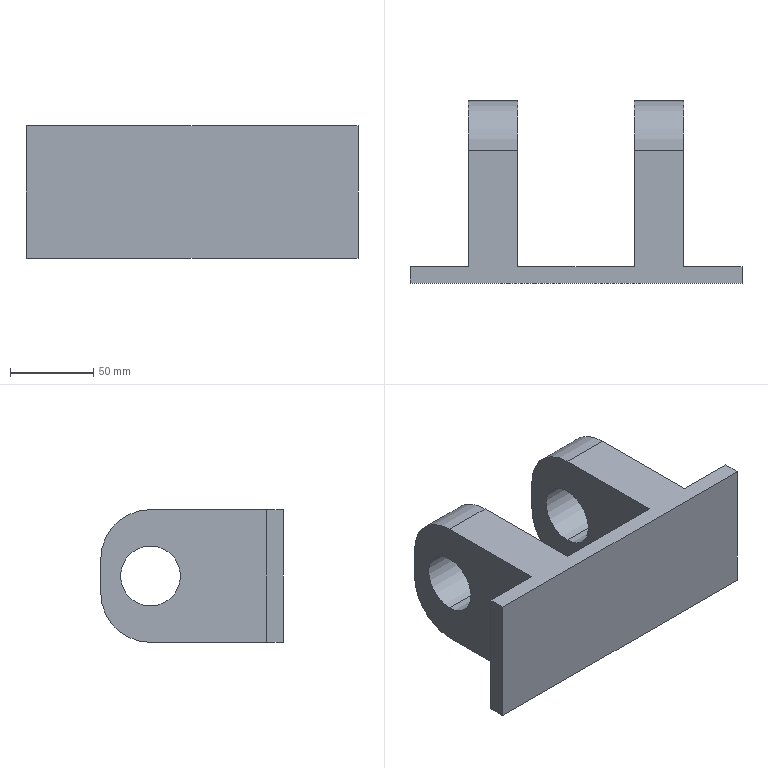Part | STEP file | Traction rod base | 1 solid | 22 faces | box 200 x 110 x 80 mm | volume 555750 mm3 | plane 14 | cylinder 8 | commonest cylinder face diameters 36 x4 60 x4
STEP:
#1=CARTESIAN_POINT('',(65.,80.,18.));
#2=VERTEX_POINT('',#1);
#3=CARTESIAN_POINT('',(65.,80.,-18.));
#4=VERTEX_POINT('',#3);
#5=CARTESIAN_POINT('',(65.,80.,0.));
#6=DIRECTION('',(1.,0.,0.));
#7=DIRECTION('',(0.,0.,-1.));
#8=AXIS2_PLACEMENT_3D('',#5,#6,#7);
#9=CIRCLE('',#8,18.);
#10=EDGE_CURVE('',#2,#4,#9,.T.);
#11=ORIENTED_EDGE('',*,*,#10,.T.);
#12=CARTESIAN_POINT('',(35.,80.,-18.));
#13=VERTEX_POINT('',#12);
#14=CARTESIAN_POINT('',(100.001,80.,-18.));
#15=DIRECTION('',(-1.,0.,0.));
#16=VECTOR('',#15,1000.);
#17=LINE('',#14,#16);
#18=EDGE_CURVE('',#4,#13,#17,.T.);
#19=ORIENTED_EDGE('',*,*,#18,.T.);
#20=CARTESIAN_POINT('',(35.,80.,18.));
#21=VERTEX_POINT('',#20);
#22=CARTESIAN_POINT('',(35.,80.,0.));
#23=DIRECTION('',(1.,0.,0.));
#24=DIRECTION('',(0.,0.,-1.));
#25=AXIS2_PLACEMENT_3D('',#22,#23,#24);
#26=CIRCLE('',#25,18.);
#27=EDGE_CURVE('',#21,#13,#26,.T.);
#28=ORIENTED_EDGE('',*,*,#27,.F.);
#29=CARTESIAN_POINT('',(100.001,80.,18.));
#30=DIRECTION('',(-1.,0.,0.));
#31=VECTOR('',#30,1000.);
#32=LINE('',#29,#31);
#33=EDGE_CURVE('',#2,#21,#32,.T.);
#34=ORIENTED_EDGE('',*,*,#33,.F.);
#35=EDGE_LOOP('',(#11,#19,#28,#34));
#36=FACE_OUTER_BOUND('',#35,.T.);
#37=CARTESIAN_POINT('',(100.001,80.,0.));
#38=DIRECTION('',(-1.,0.,0.));
#39=DIRECTION('',(0.,0.,1.));
#40=AXIS2_PLACEMENT_3D('',#37,#38,#39);
#41=CYLINDRICAL_SURFACE('',#40,18.);
#42=ADVANCED_FACE('',(#36),#41,.F.);
#43=CARTESIAN_POINT('',(-65.,80.,-18.));
#44=VERTEX_POINT('',#43);
#45=CARTESIAN_POINT('',(-65.,80.,18.));
#46=VERTEX_POINT('',#45);
#47=CARTESIAN_POINT('',(-65.,80.,0.));
#48=DIRECTION('',(-1.,0.,0.));
#49=DIRECTION('',(0.,0.,-1.));
#50=AXIS2_PLACEMENT_3D('',#47,#48,#49);
#51=CIRCLE('',#50,18.);
#52=EDGE_CURVE('',#44,#46,#51,.T.);
#53=ORIENTED_EDGE('',*,*,#52,.T.);
#54=CARTESIAN_POINT('',(-35.,80.,18.));
#55=VERTEX_POINT('',#54);
#56=CARTESIAN_POINT('',(-100.001,80.,18.));
#57=DIRECTION('',(1.,0.,0.));
#58=VECTOR('',#57,1000.);
#59=LINE('',#56,#58);
#60=EDGE_CURVE('',#46,#55,#59,.T.);
#61=ORIENTED_EDGE('',*,*,#60,.T.);
#62=CARTESIAN_POINT('',(-35.,80.,-18.));
#63=VERTEX_POINT('',#62);
#64=CARTESIAN_POINT('',(-35.,80.,0.));
#65=DIRECTION('',(1.,0.,0.));
#66=DIRECTION('',(0.,0.,-1.));
#67=AXIS2_PLACEMENT_3D('',#64,#65,#66);
#68=CIRCLE('',#67,18.);
#69=EDGE_CURVE('',#55,#63,#68,.T.);
#70=ORIENTED_EDGE('',*,*,#69,.T.);
#71=CARTESIAN_POINT('',(-100.001,80.,-18.));
#72=DIRECTION('',(1.,0.,0.));
#73=VECTOR('',#72,1000.);
#74=LINE('',#71,#73);
#75=EDGE_CURVE('',#44,#63,#74,.T.);
#76=ORIENTED_EDGE('',*,*,#75,.F.);
#77=EDGE_LOOP('',(#53,#61,#70,#76));
#78=FACE_OUTER_BOUND('',#77,.T.);
#79=CARTESIAN_POINT('',(-100.001,80.,0.));
#80=DIRECTION('',(1.,0.,0.));
#81=DIRECTION('',(0.,0.,-1.));
#82=AXIS2_PLACEMENT_3D('',#79,#80,#81);
#83=CYLINDRICAL_SURFACE('',#82,18.);
#84=ADVANCED_FACE('',(#78),#83,.F.);
#85=CARTESIAN_POINT('',(65.,10.,-40.));
#86=VERTEX_POINT('',#85);
#87=CARTESIAN_POINT('',(65.,10.,40.));
#88=VERTEX_POINT('',#87);
#89=CARTESIAN_POINT('',(65.,10.,-40.));
#90=DIRECTION('',(0.,0.,1.));
#91=VECTOR('',#90,1000.);
#92=LINE('',#89,#91);
#93=EDGE_CURVE('',#86,#88,#92,.T.);
#94=ORIENTED_EDGE('',*,*,#93,.T.);
#95=CARTESIAN_POINT('',(100.,10.,40.));
#96=VERTEX_POINT('',#95);
#97=CARTESIAN_POINT('',(-100.,10.,40.));
#98=DIRECTION('',(1.,0.,0.));
#99=VECTOR('',#98,1000.);
#100=LINE('',#97,#99);
#101=EDGE_CURVE('',#88,#96,#100,.T.);
#102=ORIENTED_EDGE('',*,*,#101,.T.);
#103=CARTESIAN_POINT('',(100.,10.,-40.));
#104=VERTEX_POINT('',#103);
#105=CARTESIAN_POINT('',(100.,10.,-40.));
#106=DIRECTION('',(0.,0.,1.));
#107=VECTOR('',#106,1000.);
#108=LINE('',#105,#107);
#109=EDGE_CURVE('',#104,#96,#108,.T.);
#110=ORIENTED_EDGE('',*,*,#109,.F.);
#111=CARTESIAN_POINT('',(-100.,10.,-40.));
#112=DIRECTION('',(1.,0.,0.));
#113=VECTOR('',#112,1000.);
#114=LINE('',#111,#113);
#115=EDGE_CURVE('',#86,#104,#114,.T.);
#116=ORIENTED_EDGE('',*,*,#115,.F.);
#117=EDGE_LOOP('',(#94,#102,#110,#116));
#118=FACE_OUTER_BOUND('',#117,.T.);
#119=CARTESIAN_POINT('',(0.,10.,0.));
#120=DIRECTION('',(0.,1.,0.));
#121=DIRECTION('',(0.,0.,1.));
#122=AXIS2_PLACEMENT_3D('',#119,#120,#121);
#123=PLANE('',#122);
#124=ADVANCED_FACE('',(#118),#123,.T.);
#125=CARTESIAN_POINT('',(-65.,10.,-40.));
#126=VERTEX_POINT('',#125);
#127=CARTESIAN_POINT('',(-65.,10.,40.));
#128=VERTEX_POINT('',#127);
#129=CARTESIAN_POINT('',(-65.,10.,-40.));
#130=DIRECTION('',(0.,0.,1.));
#131=VECTOR('',#130,1000.);
#132=LINE('',#129,#131);
#133=EDGE_CURVE('',#126,#128,#132,.T.);
#134=ORIENTED_EDGE('',*,*,#133,.F.);
#135=CARTESIAN_POINT('',(-100.,10.,-40.));
#136=VERTEX_POINT('',#135);
#137=CARTESIAN_POINT('',(-100.,10.,-40.));
#138=DIRECTION('',(1.,0.,0.));
#139=VECTOR('',#138,1000.);
#140=LINE('',#137,#139);
#141=EDGE_CURVE('',#136,#126,#140,.T.);
#142=ORIENTED_EDGE('',*,*,#141,.F.);
#143=CARTESIAN_POINT('',(-100.,10.,40.));
#144=VERTEX_POINT('',#143);
#145=CARTESIAN_POINT('',(-100.,10.,-40.));
#146=DIRECTION('',(0.,0.,1.));
#147=VECTOR('',#146,1000.);
#148=LINE('',#145,#147);
#149=EDGE_CURVE('',#136,#144,#148,.T.);
#150=ORIENTED_EDGE('',*,*,#149,.T.);
#151=CARTESIAN_POINT('',(-100.,10.,40.));
#152=DIRECTION('',(1.,0.,0.));
#153=VECTOR('',#152,1000.);
#154=LINE('',#151,#153);
#155=EDGE_CURVE('',#144,#128,#154,.T.);
#156=ORIENTED_EDGE('',*,*,#155,.T.);
#157=EDGE_LOOP('',(#134,#142,#150,#156));
#158=FACE_OUTER_BOUND('',#157,.T.);
#159=CARTESIAN_POINT('',(0.,10.,0.));
#160=DIRECTION('',(0.,1.,0.));
#161=DIRECTION('',(0.,0.,1.));
#162=AXIS2_PLACEMENT_3D('',#159,#160,#161);
#163=PLANE('',#162);
#164=ADVANCED_FACE('',(#158),#163,.T.);
#165=CARTESIAN_POINT('',(-100.,0.,-40.));
#166=VERTEX_POINT('',#165);
#167=CARTESIAN_POINT('',(-100.,0.,40.));
#168=VERTEX_POINT('',#167);
#169=CARTESIAN_POINT('',(-100.,0.,-40.));
#170=DIRECTION('',(0.,0.,1.));
#171=VECTOR('',#170,1000.);
#172=LINE('',#169,#171);
#173=EDGE_CURVE('',#166,#168,#172,.T.);
#174=ORIENTED_EDGE('',*,*,#173,.T.);
#175=CARTESIAN_POINT('',(-100.,10.,40.));
#176=DIRECTION('',(0.,-1.,0.));
#177=VECTOR('',#176,1000.);
#178=LINE('',#175,#177);
#179=EDGE_CURVE('',#144,#168,#178,.T.);
#180=ORIENTED_EDGE('',*,*,#179,.F.);
#181=ORIENTED_EDGE('',*,*,#149,.F.);
#182=CARTESIAN_POINT('',(-100.,10.,-40.));
#183=DIRECTION('',(0.,-1.,0.));
#184=VECTOR('',#183,1000.);
#185=LINE('',#182,#184);
#186=EDGE_CURVE('',#136,#166,#185,.T.);
#187=ORIENTED_EDGE('',*,*,#186,.T.);
#188=EDGE_LOOP('',(#174,#180,#181,#187));
#189=FACE_OUTER_BOUND('',#188,.T.);
#190=CARTESIAN_POINT('',(-100.,10.,-40.));
#191=DIRECTION('',(1.,0.,0.));
#192=DIRECTION('',(0.,0.,-1.));
#193=AXIS2_PLACEMENT_3D('',#190,#191,#192);
#194=PLANE('',#193);
#195=ADVANCED_FACE('',(#189),#194,.F.);
#196=CARTESIAN_POINT('',(65.,80.,40.));
#197=VERTEX_POINT('',#196);
#198=CARTESIAN_POINT('',(65.,110.,40.));
#199=DIRECTION('',(0.,-1.,0.));
#200=VECTOR('',#199,1000.);
#201=LINE('',#198,#200);
#202=EDGE_CURVE('',#197,#88,#201,.T.);
#203=ORIENTED_EDGE('',*,*,#202,.F.);
#204=CARTESIAN_POINT('',(35.,80.,40.));
#205=VERTEX_POINT('',#204);
#206=CARTESIAN_POINT('',(35.,80.,40.));
#207=DIRECTION('',(-1.,0.,0.));
#208=VECTOR('',#207,1000.);
#209=LINE('',#206,#208);
#210=EDGE_CURVE('',#197,#205,#209,.T.);
#211=ORIENTED_EDGE('',*,*,#210,.T.);
#212=CARTESIAN_POINT('',(35.,10.,40.));
#213=VERTEX_POINT('',#212);
#214=CARTESIAN_POINT('',(35.,110.,40.));
#215=DIRECTION('',(0.,-1.,0.));
#216=VECTOR('',#215,1000.);
#217=LINE('',#214,#216);
#218=EDGE_CURVE('',#205,#213,#217,.T.);
#219=ORIENTED_EDGE('',*,*,#218,.T.);
#220=CARTESIAN_POINT('',(-35.,10.,40.));
#221=VERTEX_POINT('',#220);
#222=CARTESIAN_POINT('',(-100.,10.,40.));
#223=DIRECTION('',(1.,0.,0.));
#224=VECTOR('',#223,1000.);
#225=LINE('',#222,#224);
#226=EDGE_CURVE('',#221,#213,#225,.T.);
#227=ORIENTED_EDGE('',*,*,#226,.F.);
#228=CARTESIAN_POINT('',(-35.,80.,40.));
#229=VERTEX_POINT('',#228);
#230=CARTESIAN_POINT('',(-35.,110.,40.));
#231=DIRECTION('',(0.,-1.,0.));
#232=VECTOR('',#231,1000.);
#233=LINE('',#230,#232);
#234=EDGE_CURVE('',#229,#221,#233,.T.);
#235=ORIENTED_EDGE('',*,*,#234,.F.);
#236=CARTESIAN_POINT('',(-65.,80.,40.));
#237=VERTEX_POINT('',#236);
#238=CARTESIAN_POINT('',(-65.,80.,40.));
#239=DIRECTION('',(-1.,0.,0.));
#240=VECTOR('',#239,1000.);
#241=LINE('',#238,#240);
#242=EDGE_CURVE('',#229,#237,#241,.T.);
#243=ORIENTED_EDGE('',*,*,#242,.T.);
#244=CARTESIAN_POINT('',(-65.,110.,40.));
#245=DIRECTION('',(0.,-1.,0.));
#246=VECTOR('',#245,1000.);
#247=LINE('',#244,#246);
#248=EDGE_CURVE('',#237,#128,#247,.T.);
#249=ORIENTED_EDGE('',*,*,#248,.T.);
#250=ORIENTED_EDGE('',*,*,#155,.F.);
#251=ORIENTED_EDGE('',*,*,#179,.T.);
#252=CARTESIAN_POINT('',(100.,0.,40.));
#253=VERTEX_POINT('',#252);
#254=CARTESIAN_POINT('',(-100.,0.,40.));
#255=DIRECTION('',(1.,0.,0.));
#256=VECTOR('',#255,1000.);
#257=LINE('',#254,#256);
#258=EDGE_CURVE('',#168,#253,#257,.T.);
#259=ORIENTED_EDGE('',*,*,#258,.T.);
#260=CARTESIAN_POINT('',(100.,10.,40.));
#261=DIRECTION('',(0.,-1.,0.));
#262=VECTOR('',#261,1000.);
#263=LINE('',#260,#262);
#264=EDGE_CURVE('',#96,#253,#263,.T.);
#265=ORIENTED_EDGE('',*,*,#264,.F.);
#266=ORIENTED_EDGE('',*,*,#101,.F.);
#267=EDGE_LOOP('',(#203,#211,#219,#227,#235,#243,#249,#250,#251,#259,#265,#266));
#268=FACE_OUTER_BOUND('',#267,.T.);
#269=CARTESIAN_POINT('',(-100.,10.,40.));
#270=DIRECTION('',(0.,0.,-1.));
#271=DIRECTION('',(-1.,0.,0.));
#272=AXIS2_PLACEMENT_3D('',#269,#270,#271);
#273=PLANE('',#272);
#274=ADVANCED_FACE('',(#268),#273,.F.);
#275=CARTESIAN_POINT('',(100.,0.,-40.));
#276=VERTEX_POINT('',#275);
#277=CARTESIAN_POINT('',(100.,0.,-40.));
#278=DIRECTION('',(0.,0.,1.));
#279=VECTOR('',#278,1000.);
#280=LINE('',#277,#279);
#281=EDGE_CURVE('',#276,#253,#280,.T.);
#282=ORIENTED_EDGE('',*,*,#281,.F.);
#283=CARTESIAN_POINT('',(100.,10.,-40.));
#284=DIRECTION('',(0.,-1.,0.));
#285=VECTOR('',#284,1000.);
#286=LINE('',#283,#285);
#287=EDGE_CURVE('',#104,#276,#286,.T.);
#288=ORIENTED_EDGE('',*,*,#287,.F.);
#289=ORIENTED_EDGE('',*,*,#109,.T.);
#290=ORIENTED_EDGE('',*,*,#264,.T.);
#291=EDGE_LOOP('',(#282,#288,#289,#290));
#292=FACE_OUTER_BOUND('',#291,.T.);
#293=CARTESIAN_POINT('',(100.,10.,-40.));
#294=DIRECTION('',(1.,0.,0.));
#295=DIRECTION('',(0.,0.,-1.));
#296=AXIS2_PLACEMENT_3D('',#293,#294,#295);
#297=PLANE('',#296);
#298=ADVANCED_FACE('',(#292),#297,.T.);
#299=CARTESIAN_POINT('',(35.,80.,-40.));
#300=VERTEX_POINT('',#299);
#301=CARTESIAN_POINT('',(35.,10.,-40.));
#302=VERTEX_POINT('',#301);
#303=CARTESIAN_POINT('',(35.,110.,-40.));
#304=DIRECTION('',(0.,-1.,0.));
#305=VECTOR('',#304,1000.);
#306=LINE('',#303,#305);
#307=EDGE_CURVE('',#300,#302,#306,.T.);
#308=ORIENTED_EDGE('',*,*,#307,.F.);
#309=CARTESIAN_POINT('',(65.,80.,-40.));
#310=VERTEX_POINT('',#309);
#311=CARTESIAN_POINT('',(-100.,80.,-40.));
#312=DIRECTION('',(1.,0.,0.));
#313=VECTOR('',#312,1000.);
#314=LINE('',#311,#313);
#315=EDGE_CURVE('',#300,#310,#314,.T.);
#316=ORIENTED_EDGE('',*,*,#315,.T.);
#317=CARTESIAN_POINT('',(65.,110.,-40.));
#318=DIRECTION('',(0.,-1.,0.));
#319=VECTOR('',#318,1000.);
#320=LINE('',#317,#319);
#321=EDGE_CURVE('',#310,#86,#320,.T.);
#322=ORIENTED_EDGE('',*,*,#321,.T.);
#323=ORIENTED_EDGE('',*,*,#115,.T.);
#324=ORIENTED_EDGE('',*,*,#287,.T.);
#325=CARTESIAN_POINT('',(-100.,0.,-40.));
#326=DIRECTION('',(1.,0.,0.));
#327=VECTOR('',#326,1000.);
#328=LINE('',#325,#327);
#329=EDGE_CURVE('',#166,#276,#328,.T.);
#330=ORIENTED_EDGE('',*,*,#329,.F.);
#331=ORIENTED_EDGE('',*,*,#186,.F.);
#332=ORIENTED_EDGE('',*,*,#141,.T.);
#333=CARTESIAN_POINT('',(-65.,80.,-40.));
#334=VERTEX_POINT('',#333);
#335=CARTESIAN_POINT('',(-65.,110.,-40.));
#336=DIRECTION('',(0.,-1.,0.));
#337=VECTOR('',#336,1000.);
#338=LINE('',#335,#337);
#339=EDGE_CURVE('',#334,#126,#338,.T.);
#340=ORIENTED_EDGE('',*,*,#339,.F.);
#341=CARTESIAN_POINT('',(-35.,80.,-40.));
#342=VERTEX_POINT('',#341);
#343=CARTESIAN_POINT('',(-100.,80.,-40.));
#344=DIRECTION('',(1.,0.,0.));
#345=VECTOR('',#344,1000.);
#346=LINE('',#343,#345);
#347=EDGE_CURVE('',#334,#342,#346,.T.);
#348=ORIENTED_EDGE('',*,*,#347,.T.);
#349=CARTESIAN_POINT('',(-35.,10.,-40.));
#350=VERTEX_POINT('',#349);
#351=CARTESIAN_POINT('',(-35.,110.,-40.));
#352=DIRECTION('',(0.,-1.,0.));
#353=VECTOR('',#352,1000.);
#354=LINE('',#351,#353);
#355=EDGE_CURVE('',#342,#350,#354,.T.);
#356=ORIENTED_EDGE('',*,*,#355,.T.);
#357=CARTESIAN_POINT('',(-100.,10.,-40.));
#358=DIRECTION('',(1.,0.,0.));
#359=VECTOR('',#358,1000.);
#360=LINE('',#357,#359);
#361=EDGE_CURVE('',#350,#302,#360,.T.);
#362=ORIENTED_EDGE('',*,*,#361,.T.);
#363=EDGE_LOOP('',(#308,#316,#322,#323,#324,#330,#331,#332,#340,#348,#356,#362));
#364=FACE_OUTER_BOUND('',#363,.T.);
#365=CARTESIAN_POINT('',(-100.,10.,-40.));
#366=DIRECTION('',(0.,0.,-1.));
#367=DIRECTION('',(-1.,0.,0.));
#368=AXIS2_PLACEMENT_3D('',#365,#366,#367);
#369=PLANE('',#368);
#370=ADVANCED_FACE('',(#364),#369,.T.);
#371=CARTESIAN_POINT('',(35.,10.,-40.));
#372=DIRECTION('',(0.,0.,-1.));
#373=VECTOR('',#372,1000.);
#374=LINE('',#371,#373);
#375=EDGE_CURVE('',#213,#302,#374,.T.);
#376=ORIENTED_EDGE('',*,*,#375,.T.);
#377=ORIENTED_EDGE('',*,*,#361,.F.);
#378=CARTESIAN_POINT('',(-35.,10.,-40.));
#379=DIRECTION('',(0.,0.,-1.));
#380=VECTOR('',#379,1000.);
#381=LINE('',#378,#380);
#382=EDGE_CURVE('',#221,#350,#381,.T.);
#383=ORIENTED_EDGE('',*,*,#382,.F.);
#384=ORIENTED_EDGE('',*,*,#226,.T.);
#385=EDGE_LOOP('',(#376,#377,#383,#384));
#386=FACE_OUTER_BOUND('',#385,.T.);
#387=CARTESIAN_POINT('',(0.,10.,0.));
#388=DIRECTION('',(0.,1.,0.));
#389=DIRECTION('',(0.,0.,1.));
#390=AXIS2_PLACEMENT_3D('',#387,#388,#389);
#391=PLANE('',#390);
#392=ADVANCED_FACE('',(#386),#391,.T.);
#393=ORIENTED_EDGE('',*,*,#173,.F.);
#394=ORIENTED_EDGE('',*,*,#329,.T.);
#395=ORIENTED_EDGE('',*,*,#281,.T.);
#396=ORIENTED_EDGE('',*,*,#258,.F.);
#397=EDGE_LOOP('',(#393,#394,#395,#396));
#398=FACE_OUTER_BOUND('',#397,.T.);
#399=CARTESIAN_POINT('',(0.,0.,0.));
#400=DIRECTION('',(0.,1.,0.));
#401=DIRECTION('',(0.,0.,1.));
#402=AXIS2_PLACEMENT_3D('',#399,#400,#401);
#403=PLANE('',#402);
#404=ADVANCED_FACE('',(#398),#403,.F.);
#405=ORIENTED_EDGE('',*,*,#52,.F.);
#406=CARTESIAN_POINT('',(-65.,80.,0.));
#407=DIRECTION('',(-1.,0.,0.));
#408=DIRECTION('',(0.,0.,-1.));
#409=AXIS2_PLACEMENT_3D('',#406,#407,#408);
#410=CIRCLE('',#409,18.);
#411=EDGE_CURVE('',#46,#44,#410,.T.);
#412=ORIENTED_EDGE('',*,*,#411,.F.);
#413=EDGE_LOOP('',(#405,#412));
#414=FACE_BOUND('',#413,.T.);
#415=CARTESIAN_POINT('',(-65.,110.,-10.));
#416=VERTEX_POINT('',#415);
#417=CARTESIAN_POINT('',(-65.,110.,10.));
#418=VERTEX_POINT('',#417);
#419=CARTESIAN_POINT('',(-65.,110.,-40.));
#420=DIRECTION('',(0.,0.,1.));
#421=VECTOR('',#420,1000.);
#422=LINE('',#419,#421);
#423=EDGE_CURVE('',#416,#418,#422,.T.);
#424=ORIENTED_EDGE('',*,*,#423,.F.);
#425=CARTESIAN_POINT('',(-65.,80.,-10.));
#426=DIRECTION('',(-1.,0.,0.));
#427=DIRECTION('',(0.,0.,-1.));
#428=AXIS2_PLACEMENT_3D('',#425,#426,#427);
#429=CIRCLE('',#428,30.);
#430=EDGE_CURVE('',#416,#334,#429,.T.);
#431=ORIENTED_EDGE('',*,*,#430,.T.);
#432=ORIENTED_EDGE('',*,*,#339,.T.);
#433=ORIENTED_EDGE('',*,*,#133,.T.);
#434=ORIENTED_EDGE('',*,*,#248,.F.);
#435=CARTESIAN_POINT('',(-65.,80.,10.));
#436=DIRECTION('',(-1.,0.,0.));
#437=DIRECTION('',(0.,0.,-1.));
#438=AXIS2_PLACEMENT_3D('',#435,#436,#437);
#439=CIRCLE('',#438,30.);
#440=EDGE_CURVE('',#237,#418,#439,.T.);
#441=ORIENTED_EDGE('',*,*,#440,.T.);
#442=EDGE_LOOP('',(#424,#431,#432,#433,#434,#441));
#443=FACE_OUTER_BOUND('',#442,.T.);
#444=CARTESIAN_POINT('',(-65.,110.,-40.));
#445=DIRECTION('',(1.,0.,0.));
#446=DIRECTION('',(0.,0.,-1.));
#447=AXIS2_PLACEMENT_3D('',#444,#445,#446);
#448=PLANE('',#447);
#449=ADVANCED_FACE('',(#414,#443),#448,.F.);
#450=CARTESIAN_POINT('',(-35.,80.,0.));
#451=DIRECTION('',(1.,0.,0.));
#452=DIRECTION('',(0.,0.,-1.));
#453=AXIS2_PLACEMENT_3D('',#450,#451,#452);
#454=CIRCLE('',#453,18.);
#455=EDGE_CURVE('',#63,#55,#454,.T.);
#456=ORIENTED_EDGE('',*,*,#455,.F.);
#457=ORIENTED_EDGE('',*,*,#69,.F.);
#458=EDGE_LOOP('',(#456,#457));
#459=FACE_BOUND('',#458,.T.);
#460=ORIENTED_EDGE('',*,*,#355,.F.);
#461=CARTESIAN_POINT('',(-35.,110.,-10.));
#462=VERTEX_POINT('',#461);
#463=CARTESIAN_POINT('',(-35.,80.,-10.));
#464=DIRECTION('',(1.,0.,0.));
#465=DIRECTION('',(0.,0.,1.));
#466=AXIS2_PLACEMENT_3D('',#463,#464,#465);
#467=CIRCLE('',#466,30.);
#468=EDGE_CURVE('',#342,#462,#467,.T.);
#469=ORIENTED_EDGE('',*,*,#468,.T.);
#470=CARTESIAN_POINT('',(-35.,110.,10.));
#471=VERTEX_POINT('',#470);
#472=CARTESIAN_POINT('',(-35.,110.,-40.));
#473=DIRECTION('',(0.,0.,-1.));
#474=VECTOR('',#473,1000.);
#475=LINE('',#472,#474);
#476=EDGE_CURVE('',#471,#462,#475,.T.);
#477=ORIENTED_EDGE('',*,*,#476,.F.);
#478=CARTESIAN_POINT('',(-35.,80.,10.));
#479=DIRECTION('',(1.,0.,0.));
#480=DIRECTION('',(0.,0.,1.));
#481=AXIS2_PLACEMENT_3D('',#478,#479,#480);
#482=CIRCLE('',#481,30.);
#483=EDGE_CURVE('',#471,#229,#482,.T.);
#484=ORIENTED_EDGE('',*,*,#483,.T.);
#485=ORIENTED_EDGE('',*,*,#234,.T.);
#486=ORIENTED_EDGE('',*,*,#382,.T.);
#487=EDGE_LOOP('',(#460,#469,#477,#484,#485,#486));
#488=FACE_OUTER_BOUND('',#487,.T.);
#489=CARTESIAN_POINT('',(-35.,110.,-40.));
#490=DIRECTION('',(-1.,0.,0.));
#491=DIRECTION('',(0.,0.,1.));
#492=AXIS2_PLACEMENT_3D('',#489,#490,#491);
#493=PLANE('',#492);
#494=ADVANCED_FACE('',(#459,#488),#493,.F.);
#495=ORIENTED_EDGE('',*,*,#476,.T.);
#496=CARTESIAN_POINT('',(0.,110.,-10.));
#497=DIRECTION('',(-1.,0.,0.));
#498=VECTOR('',#497,1000.);
#499=LINE('',#496,#498);
#500=EDGE_CURVE('',#462,#416,#499,.T.);
#501=ORIENTED_EDGE('',*,*,#500,.T.);
#502=ORIENTED_EDGE('',*,*,#423,.T.);
#503=CARTESIAN_POINT('',(-35.,110.,10.));
#504=DIRECTION('',(1.,0.,0.));
#505=VECTOR('',#504,1000.);
#506=LINE('',#503,#505);
#507=EDGE_CURVE('',#418,#471,#506,.T.);
#508=ORIENTED_EDGE('',*,*,#507,.T.);
#509=EDGE_LOOP('',(#495,#501,#502,#508));
#510=FACE_OUTER_BOUND('',#509,.T.);
#511=CARTESIAN_POINT('',(0.,110.,0.));
#512=DIRECTION('',(0.,1.,0.));
#513=DIRECTION('',(0.,0.,1.));
#514=AXIS2_PLACEMENT_3D('',#511,#512,#513);
#515=PLANE('',#514);
#516=ADVANCED_FACE('',(#510),#515,.T.);
#517=ORIENTED_EDGE('',*,*,#468,.F.);
#518=ORIENTED_EDGE('',*,*,#347,.F.);
#519=ORIENTED_EDGE('',*,*,#430,.F.);
#520=ORIENTED_EDGE('',*,*,#500,.F.);
#521=EDGE_LOOP('',(#517,#518,#519,#520));
#522=FACE_OUTER_BOUND('',#521,.T.);
#523=CARTESIAN_POINT('',(0.,80.,-10.));
#524=DIRECTION('',(-1.,0.,0.));
#525=DIRECTION('',(0.,0.,1.));
#526=AXIS2_PLACEMENT_3D('',#523,#524,#525);
#527=CYLINDRICAL_SURFACE('',#526,30.);
#528=ADVANCED_FACE('',(#522),#527,.T.);
#529=ORIENTED_EDGE('',*,*,#440,.F.);
#530=ORIENTED_EDGE('',*,*,#242,.F.);
#531=ORIENTED_EDGE('',*,*,#483,.F.);
#532=ORIENTED_EDGE('',*,*,#507,.F.);
#533=EDGE_LOOP('',(#529,#530,#531,#532));
#534=FACE_OUTER_BOUND('',#533,.T.);
#535=CARTESIAN_POINT('',(0.,80.,10.));
#536=DIRECTION('',(-1.,0.,0.));
#537=DIRECTION('',(0.,0.,1.));
#538=AXIS2_PLACEMENT_3D('',#535,#536,#537);
#539=CYLINDRICAL_SURFACE('',#538,30.);
#540=ADVANCED_FACE('',(#534),#539,.T.);
#541=ORIENTED_EDGE('',*,*,#60,.F.);
#542=ORIENTED_EDGE('',*,*,#411,.T.);
#543=ORIENTED_EDGE('',*,*,#75,.T.);
#544=ORIENTED_EDGE('',*,*,#455,.T.);
#545=EDGE_LOOP('',(#541,#542,#543,#544));
#546=FACE_OUTER_BOUND('',#545,.T.);
#547=CARTESIAN_POINT('',(-100.001,80.,0.));
#548=DIRECTION('',(1.,0.,0.));
#549=DIRECTION('',(0.,0.,-1.));
#550=AXIS2_PLACEMENT_3D('',#547,#548,#549);
#551=CYLINDRICAL_SURFACE('',#550,18.);
#552=ADVANCED_FACE('',(#546),#551,.F.);
#553=ORIENTED_EDGE('',*,*,#10,.F.);
#554=CARTESIAN_POINT('',(65.,80.,0.));
#555=DIRECTION('',(1.,0.,0.));
#556=DIRECTION('',(0.,0.,-1.));
#557=AXIS2_PLACEMENT_3D('',#554,#555,#556);
#558=CIRCLE('',#557,18.);
#559=EDGE_CURVE('',#4,#2,#558,.T.);
#560=ORIENTED_EDGE('',*,*,#559,.F.);
#561=EDGE_LOOP('',(#553,#560));
#562=FACE_BOUND('',#561,.T.);
#563=ORIENTED_EDGE('',*,*,#321,.F.);
#564=CARTESIAN_POINT('',(65.,110.,-10.));
#565=VERTEX_POINT('',#564);
#566=CARTESIAN_POINT('',(65.,80.,-10.));
#567=DIRECTION('',(1.,0.,0.));
#568=DIRECTION('',(0.,0.,-1.));
#569=AXIS2_PLACEMENT_3D('',#566,#567,#568);
#570=CIRCLE('',#569,30.);
#571=EDGE_CURVE('',#310,#565,#570,.T.);
#572=ORIENTED_EDGE('',*,*,#571,.T.);
#573=CARTESIAN_POINT('',(65.,110.,10.));
#574=VERTEX_POINT('',#573);
#575=CARTESIAN_POINT('',(65.,110.,-40.));
#576=DIRECTION('',(0.,0.,1.));
#577=VECTOR('',#576,1000.);
#578=LINE('',#575,#577);
#579=EDGE_CURVE('',#565,#574,#578,.T.);
#580=ORIENTED_EDGE('',*,*,#579,.T.);
#581=CARTESIAN_POINT('',(65.,80.,10.));
#582=DIRECTION('',(1.,0.,0.));
#583=DIRECTION('',(0.,0.,-1.));
#584=AXIS2_PLACEMENT_3D('',#581,#582,#583);
#585=CIRCLE('',#584,30.);
#586=EDGE_CURVE('',#574,#197,#585,.T.);
#587=ORIENTED_EDGE('',*,*,#586,.T.);
#588=ORIENTED_EDGE('',*,*,#202,.T.);
#589=ORIENTED_EDGE('',*,*,#93,.F.);
#590=EDGE_LOOP('',(#563,#572,#580,#587,#588,#589));
#591=FACE_OUTER_BOUND('',#590,.T.);
#592=CARTESIAN_POINT('',(65.,110.,-40.));
#593=DIRECTION('',(1.,0.,0.));
#594=DIRECTION('',(0.,0.,-1.));
#595=AXIS2_PLACEMENT_3D('',#592,#593,#594);
#596=PLANE('',#595);
#597=ADVANCED_FACE('',(#562,#591),#596,.T.);
#598=ORIENTED_EDGE('',*,*,#27,.T.);
#599=CARTESIAN_POINT('',(35.,80.,0.));
#600=DIRECTION('',(1.,0.,0.));
#601=DIRECTION('',(0.,0.,-1.));
#602=AXIS2_PLACEMENT_3D('',#599,#600,#601);
#603=CIRCLE('',#602,18.);
#604=EDGE_CURVE('',#13,#21,#603,.T.);
#605=ORIENTED_EDGE('',*,*,#604,.T.);
#606=EDGE_LOOP('',(#598,#605));
#607=FACE_BOUND('',#606,.T.);
#608=CARTESIAN_POINT('',(35.,110.,10.));
#609=VERTEX_POINT('',#608);
#610=CARTESIAN_POINT('',(35.,110.,-10.));
#611=VERTEX_POINT('',#610);
#612=CARTESIAN_POINT('',(35.,110.,-40.));
#613=DIRECTION('',(0.,0.,-1.));
#614=VECTOR('',#613,1000.);
#615=LINE('',#612,#614);
#616=EDGE_CURVE('',#609,#611,#615,.T.);
#617=ORIENTED_EDGE('',*,*,#616,.T.);
#618=CARTESIAN_POINT('',(35.,80.,-10.));
#619=DIRECTION('',(-1.,0.,0.));
#620=DIRECTION('',(0.,0.,1.));
#621=AXIS2_PLACEMENT_3D('',#618,#619,#620);
#622=CIRCLE('',#621,30.);
#623=EDGE_CURVE('',#611,#300,#622,.T.);
#624=ORIENTED_EDGE('',*,*,#623,.T.);
#625=ORIENTED_EDGE('',*,*,#307,.T.);
#626=ORIENTED_EDGE('',*,*,#375,.F.);
#627=ORIENTED_EDGE('',*,*,#218,.F.);
#628=CARTESIAN_POINT('',(35.,80.,10.));
#629=DIRECTION('',(-1.,0.,0.));
#630=DIRECTION('',(0.,0.,1.));
#631=AXIS2_PLACEMENT_3D('',#628,#629,#630);
#632=CIRCLE('',#631,30.);
#633=EDGE_CURVE('',#205,#609,#632,.T.);
#634=ORIENTED_EDGE('',*,*,#633,.T.);
#635=EDGE_LOOP('',(#617,#624,#625,#626,#627,#634));
#636=FACE_OUTER_BOUND('',#635,.T.);
#637=CARTESIAN_POINT('',(35.,110.,-40.));
#638=DIRECTION('',(-1.,0.,0.));
#639=DIRECTION('',(0.,0.,1.));
#640=AXIS2_PLACEMENT_3D('',#637,#638,#639);
#641=PLANE('',#640);
#642=ADVANCED_FACE('',(#607,#636),#641,.T.);
#643=ORIENTED_EDGE('',*,*,#579,.F.);
#644=CARTESIAN_POINT('',(0.,110.,-10.));
#645=DIRECTION('',(-1.,0.,0.));
#646=VECTOR('',#645,1000.);
#647=LINE('',#644,#646);
#648=EDGE_CURVE('',#565,#611,#647,.T.);
#649=ORIENTED_EDGE('',*,*,#648,.T.);
#650=ORIENTED_EDGE('',*,*,#616,.F.);
#651=CARTESIAN_POINT('',(65.,110.,10.));
#652=DIRECTION('',(1.,0.,0.));
#653=VECTOR('',#652,1000.);
#654=LINE('',#651,#653);
#655=EDGE_CURVE('',#609,#574,#654,.T.);
#656=ORIENTED_EDGE('',*,*,#655,.T.);
#657=EDGE_LOOP('',(#643,#649,#650,#656));
#658=FACE_OUTER_BOUND('',#657,.T.);
#659=CARTESIAN_POINT('',(0.,110.,0.));
#660=DIRECTION('',(0.,1.,0.));
#661=DIRECTION('',(0.,0.,1.));
#662=AXIS2_PLACEMENT_3D('',#659,#660,#661);
#663=PLANE('',#662);
#664=ADVANCED_FACE('',(#658),#663,.T.);
#665=ORIENTED_EDGE('',*,*,#623,.F.);
#666=ORIENTED_EDGE('',*,*,#648,.F.);
#667=ORIENTED_EDGE('',*,*,#571,.F.);
#668=ORIENTED_EDGE('',*,*,#315,.F.);
#669=EDGE_LOOP('',(#665,#666,#667,#668));
#670=FACE_OUTER_BOUND('',#669,.T.);
#671=CARTESIAN_POINT('',(-100.,80.,-10.));
#672=DIRECTION('',(1.,0.,0.));
#673=DIRECTION('',(0.,0.,-1.));
#674=AXIS2_PLACEMENT_3D('',#671,#672,#673);
#675=CYLINDRICAL_SURFACE('',#674,30.);
#676=ADVANCED_FACE('',(#670),#675,.T.);
#677=ORIENTED_EDGE('',*,*,#586,.F.);
#678=ORIENTED_EDGE('',*,*,#655,.F.);
#679=ORIENTED_EDGE('',*,*,#633,.F.);
#680=ORIENTED_EDGE('',*,*,#210,.F.);
#681=EDGE_LOOP('',(#677,#678,#679,#680));
#682=FACE_OUTER_BOUND('',#681,.T.);
#683=CARTESIAN_POINT('',(-100.,80.,10.));
#684=DIRECTION('',(1.,0.,0.));
#685=DIRECTION('',(0.,0.,-1.));
#686=AXIS2_PLACEMENT_3D('',#683,#684,#685);
#687=CYLINDRICAL_SURFACE('',#686,30.);
#688=ADVANCED_FACE('',(#682),#687,.T.);
#689=ORIENTED_EDGE('',*,*,#18,.F.);
#690=ORIENTED_EDGE('',*,*,#559,.T.);
#691=ORIENTED_EDGE('',*,*,#33,.T.);
#692=ORIENTED_EDGE('',*,*,#604,.F.);
#693=EDGE_LOOP('',(#689,#690,#691,#692));
#694=FACE_OUTER_BOUND('',#693,.T.);
#695=CARTESIAN_POINT('',(100.001,80.,0.));
#696=DIRECTION('',(-1.,0.,0.));
#697=DIRECTION('',(0.,0.,1.));
#698=AXIS2_PLACEMENT_3D('',#695,#696,#697);
#699=CYLINDRICAL_SURFACE('',#698,18.);
#700=ADVANCED_FACE('',(#694),#699,.F.);
#701=CLOSED_SHELL('',(#42,#84,#124,#164,#195,#274,#298,#370,#392,#404,#449,#494,#516,#528,#540,#552,#597,#642,#664,#676,#688,#700));
#702=MANIFOLD_SOLID_BREP('',#701);
#703=CARTESIAN_POINT('',(0.,0.,0.));
#704=DIRECTION('',(0.,0.,1.));
#705=DIRECTION('',(1.,0.,0.));
#706=AXIS2_PLACEMENT_3D('',#703,#704,#705);
#707=(LENGTH_UNIT()NAMED_UNIT(*)SI_UNIT(.MILLI.,.METRE.));
#708=UNCERTAINTY_MEASURE_WITH_UNIT(LENGTH_MEASURE(0.00001),#707,'','');
#709=(NAMED_UNIT(*)PLANE_ANGLE_UNIT()SI_UNIT($,.RADIAN.));
#710=(NAMED_UNIT(*)SI_UNIT($,.STERADIAN.)SOLID_ANGLE_UNIT());
#711=(GEOMETRIC_REPRESENTATION_CONTEXT(3)GLOBAL_UNCERTAINTY_ASSIGNED_CONTEXT((#708))GLOBAL_UNIT_ASSIGNED_CONTEXT((#707,#709,#710))REPRESENTATION_CONTEXT('',''));
#712=ADVANCED_BREP_SHAPE_REPRESENTATION('',(#702,#706),#711);